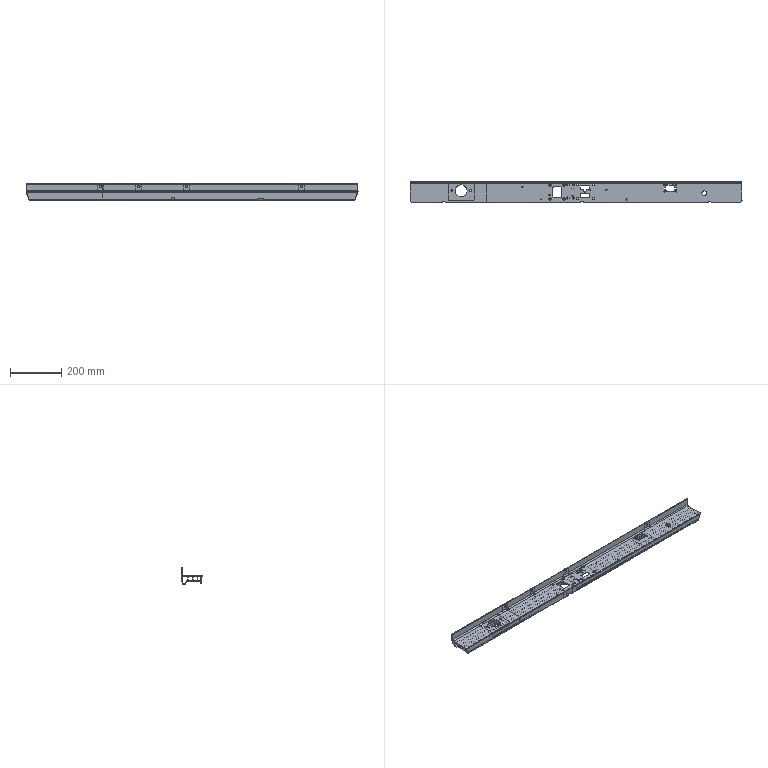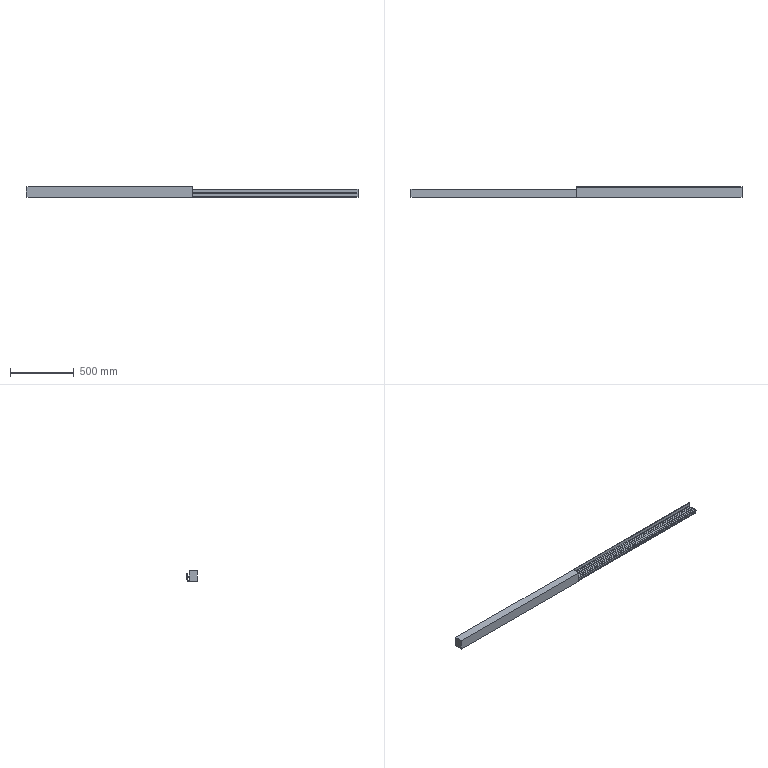CAM job | NX | 3+2 milling | part box 1301 x 81.1 x 63 mm | stock box 2601 x 81.1 x 81.1 mm
Tools:
number,name,description,diameter,corner_radius,flute_length,length,flutes
16,D16,Milling Tool-5 Parameters,16.0,0.0,50.0,75.0,2
10,D10,Milling Tool-5 Parameters,10.0,0.0,50.0,75.0,2
8,D8R0.5,Milling Tool-5 Parameters,8.0,0.5,50.0,75.0,2
6,D6,Milling Tool-5 Parameters,6.0,0.0,50.0,75.0,2
4,D4,Milling Tool-5 Parameters,4.0,0.0,50.0,75.0,2
3,D3,Milling Tool-5 Parameters,3.0,0.0,50.0,75.0,2
15,D1.5,Milling Tool-5 Parameters,1.5,0.0,50.0,75.0,2
2,D2,Milling Tool-5 Parameters,2.0,0.0,50.0,75.0,2
1,D1,Milling Tool-5 Parameters,1.0,0.0,50.0,75.0,2
7,D6A45,Milling Tool-5 Parameters,6.0,0.0,3.0,3.0,2
9,R3,Milling Tool-5 Parameters,6.0,3.0,50.0,75.0,2
Operations:
program,operation,operation_type,tool,method,geometry_group,spindle_rpm,surface_speed,feed_per_tooth,feed_cut,feed_plunge,cut_length_mm,path_length_mm,cut_time_min,machine_time_min
1,ZLEVEL_PROFILE,ZLevelMilling,D16,METHOD,MCS_MILL-A,6000.0,301.0,0.1667,2000.0,100.0,1822.353,3384.662,0.9112,1.067
1,ZLEVEL_PROFILE_COPY,ZLevelMilling,D16,METHOD,MCS_MILL-A,6000.0,301.0,0.1667,2000.0,100.0,636.682,2211.31,0.3183,0.4758
1,CAVITY_MILL,CavityMilling,D16,METHOD,A,9500.0,477.0,0.1316,2500.0,1000.0,84499.057,87972.626,35.058,35.405
1,HOLE_MILLING,CylinderMilling,D16,METHOD,A,6000.0,301.0,0.1667,2000.0,100.0,3721.874,5006.223,1.861,1.989
1,FLOOR_WALL,VolumeBased25DMillingOperation,D10,METHOD,A,6000.0,188.0,0.0833,1000.0,100.0,3586.37,5423.69,3.586,3.77
1,11,ZLevelMilling,D10,METHOD,A,5500.0,138.0,0.0909,1000.0,500.0,400.068,2351.109,0.4893,0.6845
1,FLOOR_WALL_COPY,VolumeBased25DMillingOperation,D10,METHOD,A,6000.0,188.0,0.0833,1000.0,100.0,1652.283,1769.883,1.652,1.664
1,ZLEVEL_PROFILE_COPY_2,ZLevelMilling,D10,METHOD,A,6000.0,188.0,0.1667,2000.0,1000.0,1358.992,2296.564,0.775,0.8688
1,HOLE_MILLING_1_COPY_1,CylinderMilling,D10,METHOD,A,6000.0,113.0,0.1167,1400.0,100.0,125.942,912.94,0.09,0.1687
1,ZLEVEL_PROFILE_1,ZLevelMilling,D8R0.5,METHOD,A,6000.0,150.0,0.2083,2500.0,1000.0,1765.292,3258.075,0.7231,0.8724
1,ZLEVEL_PROFILE_1_COPY,ZLevelMilling,D8R0.5,METHOD,A,6000.0,150.0,0.2083,2500.0,1000.0,3408.024,6259.7,1.393,1.678
1,HOLE_MILLING_1,CylinderMilling,D6,METHOD,A,6000.0,113.0,0.1167,1400.0,100.0,588.287,2025.847,0.4202,0.564
1,HOLE_MILLING_1_COPY,CylinderMilling,D4,METHOD,A,6000.0,113.0,0.1167,1400.0,100.0,254.337,1005.873,0.1817,0.2568
1,ZLEVEL_PROFILE_COPY_2_COPY,ZLevelMilling,D4,METHOD,A,6000.0,75.0,0.1167,1400.0,1000.0,1847.229,5659.288,1.378,1.76
1,HOLE_MILLING_1_COPY_COPY,CylinderMilling,D3,METHOD,A,6000.0,56.0,0.1,1200.0,100.0,315.457,921.258,0.2629,0.3235
1,ZLEVEL_PROFILE_COPY_2_COPY_COPY,ZLevelMilling,D2,METHOD,A,6000.0,37.0,0.0833,1000.0,1000.0,786.709,2791.034,0.7867,0.9871
1,HOLE_MILLING_1_COPY_COPY_COPY,CylinderMilling,D1.5,METHOD,A,6000.0,28.0,0.0833,1000.0,100.0,90.992,212.692,0.091,0.1032
1,ZLEVEL_PROFILE_COPY_2_COPY_COPY_COPY,ZLevelMilling,D1,METHOD,A,6000.0,18.0,0.0708,850.0,1000.0,664.555,2696.039,0.7675,0.9706
1,ZLEVEL_PROFILE_COPY_1_COPY_COPY_COPY_COPY,ZLevelMilling,D6A45,METHOD,A,6000.0,113.0,0.0833,1000.0,1000.0,919.324,6018.914,0.9193,1.429
1,刀补16,CylinderMilling,D16,METHOD,A,6000.0,301.0,0.1,1200.0,100.0,860.802,2110.352,0.7173,0.8423
1,刀补16刀补,CylinderMilling,D6,METHOD,A,6000.0,113.0,0.0833,1000.0,100.0,229.687,1667.247,0.2297,0.3734
1,刀补16刀补16,CylinderMilling,D4,METHOD,A,6000.0,113.0,0.1167,1400.0,100.0,256.237,1007.773,0.183,0.2582
1,刀补16刀补16刀补16,ZLevelMilling,D4,METHOD,A,6000.0,75.0,0.0833,1000.0,500.0,342.009,866.423,0.3549,0.4074
1,刀补16刀补16刀补16刀补16,CylinderMilling,D3,METHOD,A,6000.0,56.0,0.1,1200.0,100.0,97.003,702.804,0.0808,0.1414
1,刀补16刀补16刀补16刀补16刀补16,ZLevelMilling,D2,METHOD,A,6000.0,75.0,0.0833,1000.0,500.0,140.05,260.051,0.1437,0.1557
1,刀补16刀补16刀补16刀补16刀补16刀补16刀补16,CylinderMilling,D1.5,METHOD,A,6000.0,28.0,0.0833,1000.0,100.0,17.744,139.444,0.0177,0.0299
2,FLOOR_WALL_COPY_COPY,VolumeBased25DMillingOperation,D10,METHOD,B,6000.0,188.0,0.2083,2500.0,1000.0,78202.793,103437.318,37.485,40.008
2,FLOOR_WALL_COPY_COPY_1,VolumeBased25DMillingOperation,D10,METHOD,B,6000.0,188.0,0.0833,1000.0,100.0,3443.125,4584.863,3.443,3.557
2,ZLEVEL_PROFILE_1_COPY_1,ZLevelMilling,D8R0.5,METHOD,B,6000.0,150.0,0.2083,2500.0,1000.0,79225.801,80674.584,31.695,31.84
2,FIXED_CONTOUR_COPY,SurfaceContour,D6,METHOD,B,9500.0,179.0,0.1316,2500.0,1000.0,1448.652,1880.835,0.586,0.6292
2,FIXED_CONTOUR,SurfaceContour,R3,METHOD,B,9500.0,179.0,0.1316,2500.0,1000.0,865.161,1315.059,0.3526,0.3976
2,HOLE_MILLING_1_COPY_COPY_1,CylinderMilling,D4,METHOD,B,6000.0,113.0,0.1167,1400.0,100.0,1060.576,3496.047,0.7576,1.001
2,ZLEVEL_PROFILE_COPY_2_COPY_1,ZLevelMilling,D4,METHOD,B,6000.0,75.0,0.1167,1400.0,1000.0,632.564,1623.976,0.4825,0.5817
2,HOLE_MILLING_1_COPY_COPY_1_COPY,CylinderMilling,D3,METHOD,B,6000.0,113.0,0.1167,1400.0,100.0,248.436,1072.531,0.1775,0.2599
2,ZLEVEL_PROFILE_COPY_1_COPY_COPY_COPY_COPY_COPY,ZLevelMilling,D6A45,METHOD,B,6000.0,113.0,0.0833,1000.0,1000.0,789.049,12177.727,0.789,1.928
2,刀补10,VolumeBased25DMillingOperation,D10,METHOD,B,6000.0,188.0,0.0833,1000.0,100.0,1578.144,2352.596,1.578,1.656
2,HOLE_MILLING_1_COPY_COPY_1_COPY_1,CylinderMilling,D4,METHOD,B,6000.0,113.0,0.0833,1000.0,100.0,318.388,2550.603,0.3184,0.5416
2,HOLE_MILLING_1_COPY_COPY_1_COPY_1_COPY,CylinderMilling,D4,METHOD,B,6000.0,113.0,0.0833,1000.0,100.0,26.194,108.694,0.0262,0.0344
2,刀补16刀补16刀补16_COPY,ZLevelMilling,D4,METHOD,B,6000.0,75.0,0.0833,1000.0,500.0,83.115,1062.803,0.0954,0.1933
2,HOLE_MILLING_1_COPY_COPY_1_COPY_COPY,CylinderMilling,D3,METHOD,B,6000.0,113.0,0.0833,1000.0,100.0,250.983,1075.079,0.251,0.3334
3,HOLE_MILLING_1_COPY_2,CylinderMilling,D6,METHOD,C,6000.0,113.0,0.1167,1400.0,100.0,328.759,1369.158,0.2348,0.3389
3,ZLEVEL_PROFILE_COPY_1_COPY_COPY_COPY_COPY_COPY_1,ZLevelMilling,D6A45,METHOD,C,6000.0,113.0,0.0833,1000.0,1000.0,73.461,1116.12,0.0735,0.1777
3,刀补16刀补_COPY,CylinderMilling,D6,METHOD,C,6000.0,113.0,0.0833,1000.0,100.0,123.773,1164.172,0.1238,0.2278